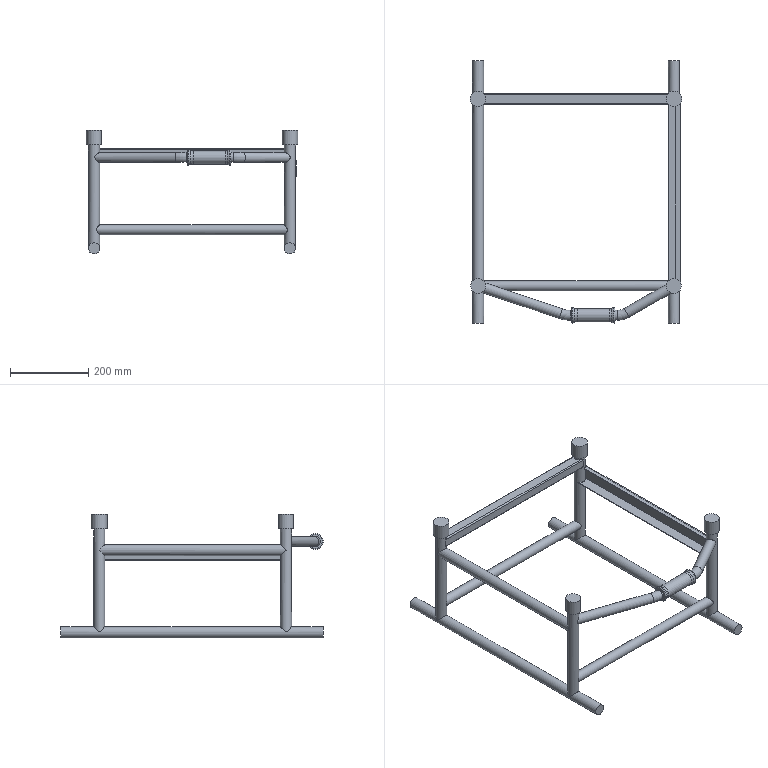Part | STEP file | DEWALT-DWE7492-B22 | 1 solid | 66 faces | box 540.27 x 670 x 316.25 mm | volume 3162222 mm3 | plane 31 | cylinder 26 | torus 6 | cone 2 | other 1 | commonest cylinder face diameters 6 x6 25.5 x6 28.4 x5 4 x3 28.5 x2 37.992 x2